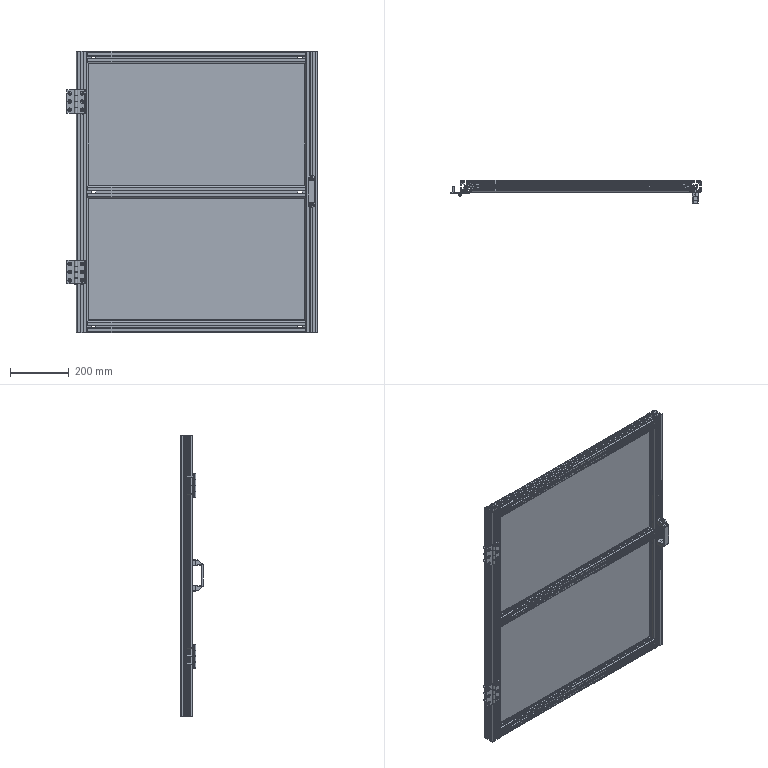Part | SolidWorks | features ReferencePattern 28, LocalLPattern 5, MirrorCompFeat 2 | 61 solids | 2656 faces | box 852 x 78 x 956 mm | volume 5159135 mm3 | plane 1738 | cylinder 707 | cone 189 | spline 22 | commonest cylinder face diameters 1.5 x66 2 x64 0.562 x60 6.8 x55 6 x40 6.5 x40